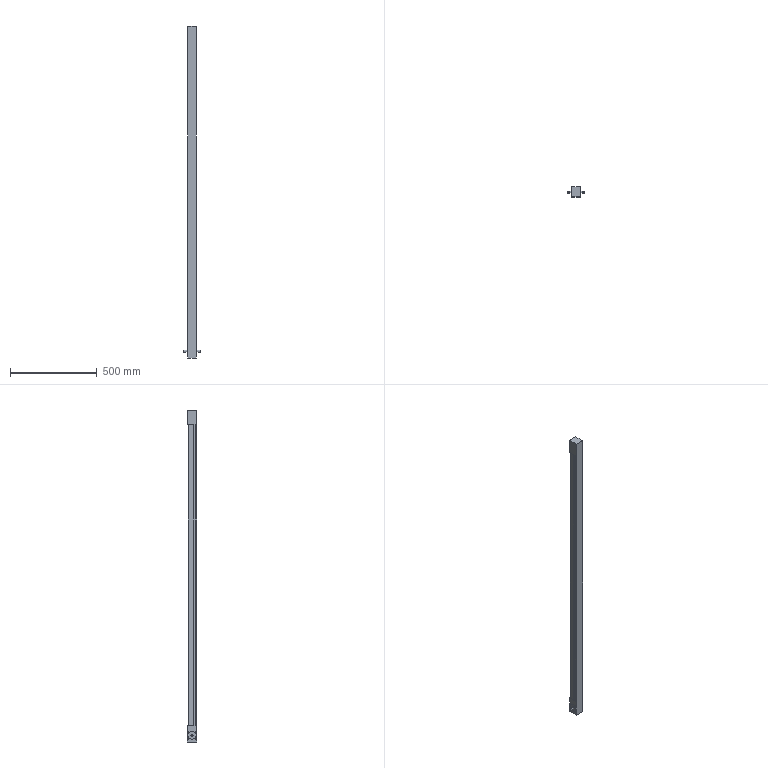Part | SolidWorks | features Boss 3, 3DProfileFeature 1, Chamfer 1, CirPattern 1, Cut 1, Extrusion 1, HoleWzd 1, MirrorPattern 1 | 1 solid | 108 faces | box 99 x 55.5 x 1910 mm | volume 4289434 mm3 | plane 50 | cylinder 40 | cone 18 | commonest cylinder face diameters 4.2 x16 5 x16 12 x4 47 x4